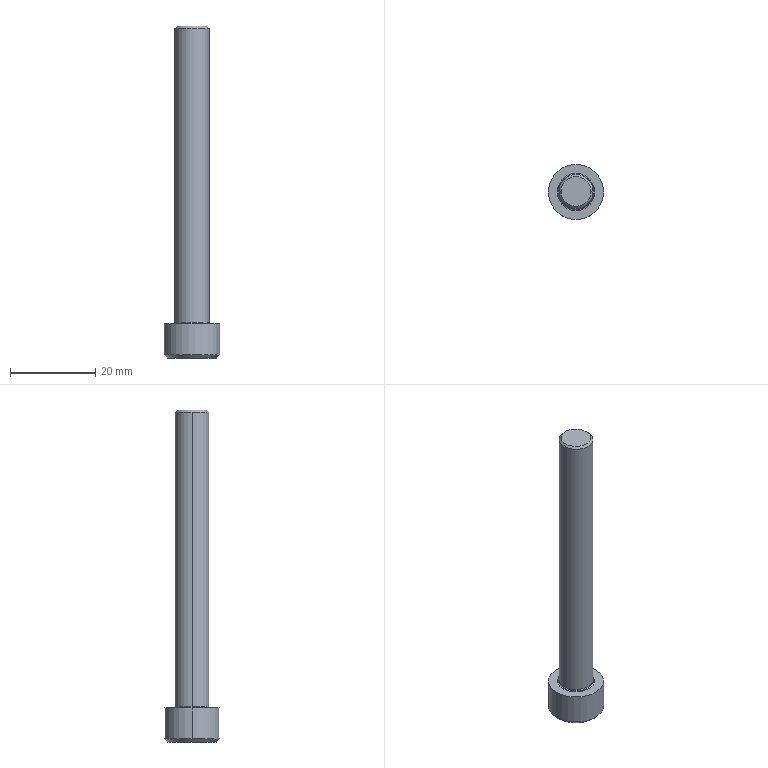Part | Creo | 1 solid | 23 faces | box 13 x 13 x 78 mm | volume 4417 mm3 | plane 9 | cone 6 | cylinder 4 | torus 4 | commonest cylinder face diameters 8 x2 13 x2
STEP:
#1=CARTESIAN_POINT('',(0.,0.,0.));
#2=DIRECTION('',(0.,0.,1.));
#3=DIRECTION('',(1.,0.,0.));
#4=AXIS2_PLACEMENT_3D('',#1,#2,#3);
#5=CARTESIAN_POINT('',(-18.464,-45.,-115.5));
#6=VERTEX_POINT('',#5);
#7=CARTESIAN_POINT('',(-16.732,-42.,-115.5));
#8=VERTEX_POINT('',#7);
#9=CARTESIAN_POINT('',(-18.464,-45.,-115.5));
#10=CARTESIAN_POINT('',(-18.409,-44.904,-115.468));
#11=CARTESIAN_POINT('',(-18.3,-44.716,-115.41));
#12=CARTESIAN_POINT('',(-18.143,-44.444,-115.34));
#13=CARTESIAN_POINT('',(-17.988,-44.176,-115.287));
#14=CARTESIAN_POINT('',(-17.834,-43.908,-115.25));
#15=CARTESIAN_POINT('',(-17.677,-43.636,-115.231));
#16=CARTESIAN_POINT('',(-17.519,-43.364,-115.231));
#17=CARTESIAN_POINT('',(-17.362,-43.092,-115.25));
#18=CARTESIAN_POINT('',(-17.208,-42.824,-115.287));
#19=CARTESIAN_POINT('',(-17.053,-42.556,-115.34));
#20=CARTESIAN_POINT('',(-16.896,-42.284,-115.41));
#21=CARTESIAN_POINT('',(-16.787,-42.096,-115.468));
#22=CARTESIAN_POINT('',(-16.732,-42.,-115.5));
#23=B_SPLINE_CURVE_WITH_KNOTS('',3,(#9,#10,#11,#12,#13,#14,#15,#16,#17,#18,#19,#20,#21,#22),.UNSPECIFIED.,.F.,.F.,(4,1,1,1,1,1,1,1,1,1,1,4),(0.,0.09091,0.1818,0.2727,0.3636,0.4545,0.5455,0.6364,0.7273,0.8182,0.9091,1.),.UNSPECIFIED.);
#24=EDGE_CURVE('',#6,#8,#23,.T.);
#25=ORIENTED_EDGE('',*,*,#24,.F.);
#26=CARTESIAN_POINT('',(-15.,-45.,-113.5));
#27=VERTEX_POINT('',#26);
#28=CARTESIAN_POINT('',(-15.,-45.,-113.5));
#29=DIRECTION('',(-0.866,0.,-0.5));
#30=VECTOR('',#29,4.);
#31=LINE('',#28,#30);
#32=EDGE_CURVE('',#27,#6,#31,.T.);
#33=ORIENTED_EDGE('',*,*,#32,.F.);
#34=CARTESIAN_POINT('',(-11.536,-45.,-115.5));
#35=VERTEX_POINT('',#34);
#36=CARTESIAN_POINT('',(-15.,-45.,-113.5));
#37=DIRECTION('',(0.866,0.,-0.5));
#38=VECTOR('',#37,4.);
#39=LINE('',#36,#38);
#40=EDGE_CURVE('',#27,#35,#39,.T.);
#41=ORIENTED_EDGE('',*,*,#40,.T.);
#42=CARTESIAN_POINT('',(-13.268,-42.,-115.5));
#43=VERTEX_POINT('',#42);
#44=CARTESIAN_POINT('',(-13.268,-42.,-115.5));
#45=CARTESIAN_POINT('',(-13.213,-42.096,-115.468));
#46=CARTESIAN_POINT('',(-13.104,-42.284,-115.41));
#47=CARTESIAN_POINT('',(-12.947,-42.556,-115.34));
#48=CARTESIAN_POINT('',(-12.792,-42.824,-115.287));
#49=CARTESIAN_POINT('',(-12.638,-43.092,-115.25));
#50=CARTESIAN_POINT('',(-12.481,-43.364,-115.231));
#51=CARTESIAN_POINT('',(-12.323,-43.636,-115.231));
#52=CARTESIAN_POINT('',(-12.166,-43.908,-115.25));
#53=CARTESIAN_POINT('',(-12.012,-44.176,-115.287));
#54=CARTESIAN_POINT('',(-11.857,-44.444,-115.34));
#55=CARTESIAN_POINT('',(-11.7,-44.716,-115.41));
#56=CARTESIAN_POINT('',(-11.591,-44.904,-115.468));
#57=CARTESIAN_POINT('',(-11.536,-45.,-115.5));
#58=B_SPLINE_CURVE_WITH_KNOTS('',3,(#44,#45,#46,#47,#48,#49,#50,#51,#52,#53,#54,#55,#56,#57),.UNSPECIFIED.,.F.,.F.,(4,1,1,1,1,1,1,1,1,1,1,4),(0.,0.09091,0.1818,0.2727,0.3636,0.4545,0.5455,0.6364,0.7273,0.8182,0.9091,1.),.UNSPECIFIED.);
#59=EDGE_CURVE('',#43,#35,#58,.T.);
#60=ORIENTED_EDGE('',*,*,#59,.F.);
#61=CARTESIAN_POINT('',(-16.732,-42.,-115.5));
#62=CARTESIAN_POINT('',(-16.622,-42.,-115.468));
#63=CARTESIAN_POINT('',(-16.404,-42.,-115.41));
#64=CARTESIAN_POINT('',(-16.091,-42.,-115.34));
#65=CARTESIAN_POINT('',(-15.782,-42.,-115.287));
#66=CARTESIAN_POINT('',(-15.472,-42.,-115.25));
#67=CARTESIAN_POINT('',(-15.158,-42.,-115.231));
#68=CARTESIAN_POINT('',(-14.842,-42.,-115.231));
#69=CARTESIAN_POINT('',(-14.528,-42.,-115.25));
#70=CARTESIAN_POINT('',(-14.218,-42.,-115.287));
#71=CARTESIAN_POINT('',(-13.909,-42.,-115.34));
#72=CARTESIAN_POINT('',(-13.596,-42.,-115.41));
#73=CARTESIAN_POINT('',(-13.378,-42.,-115.468));
#74=CARTESIAN_POINT('',(-13.268,-42.,-115.5));
#75=B_SPLINE_CURVE_WITH_KNOTS('',3,(#61,#62,#63,#64,#65,#66,#67,#68,#69,#70,#71,#72,#73,#74),.UNSPECIFIED.,.F.,.F.,(4,1,1,1,1,1,1,1,1,1,1,4),(0.,0.09091,0.1818,0.2727,0.3636,0.4545,0.5455,0.6364,0.7273,0.8182,0.9091,1.),.UNSPECIFIED.);
#76=EDGE_CURVE('',#8,#43,#75,.T.);
#77=ORIENTED_EDGE('',*,*,#76,.F.);
#78=EDGE_LOOP('',(#25,#33,#41,#60,#77));
#79=FACE_OUTER_BOUND('',#78,.F.);
#80=CARTESIAN_POINT('',(-15.,-45.,-114.524));
#81=DIRECTION('',(0.,0.,-1.));
#82=DIRECTION('',(-1.,0.,0.));
#83=AXIS2_PLACEMENT_3D('',#80,#81,#82);
#84=CONICAL_SURFACE('',#83,1.774,60.);
#85=ADVANCED_FACE('',(#79),#84,.F.);
#86=CARTESIAN_POINT('',(-16.732,-42.,-119.5));
#87=VERTEX_POINT('',#86);
#88=CARTESIAN_POINT('',(-18.464,-45.,-119.5));
#89=VERTEX_POINT('',#88);
#90=CARTESIAN_POINT('',(-16.732,-42.,-119.5));
#91=DIRECTION('',(-0.5,-0.866,0.));
#92=VECTOR('',#91,3.464);
#93=LINE('',#90,#92);
#94=EDGE_CURVE('',#87,#89,#93,.T.);
#95=ORIENTED_EDGE('',*,*,#94,.T.);
#96=CARTESIAN_POINT('',(-18.464,-45.,-119.5));
#97=DIRECTION('',(0.,0.,1.));
#98=VECTOR('',#97,4.);
#99=LINE('',#96,#98);
#100=EDGE_CURVE('',#89,#6,#99,.T.);
#101=ORIENTED_EDGE('',*,*,#100,.T.);
#102=ORIENTED_EDGE('',*,*,#24,.T.);
#103=CARTESIAN_POINT('',(-16.732,-42.,-119.5));
#104=DIRECTION('',(0.,0.,1.));
#105=VECTOR('',#104,4.);
#106=LINE('',#103,#105);
#107=EDGE_CURVE('',#87,#8,#106,.T.);
#108=ORIENTED_EDGE('',*,*,#107,.F.);
#109=EDGE_LOOP('',(#95,#101,#102,#108));
#110=FACE_OUTER_BOUND('',#109,.F.);
#111=CARTESIAN_POINT('',(-16.732,-42.,-115.5));
#112=DIRECTION('',(0.866,-0.5,0.));
#113=DIRECTION('',(-0.5,-0.866,0.));
#114=AXIS2_PLACEMENT_3D('',#111,#112,#113);
#115=PLANE('',#114);
#116=ADVANCED_FACE('',(#110),#115,.T.);
#117=CARTESIAN_POINT('',(-20.7,-45.,-119.5));
#118=VERTEX_POINT('',#117);
#119=CARTESIAN_POINT('',(-9.3,-45.,-119.5));
#120=VERTEX_POINT('',#119);
#121=CARTESIAN_POINT('',(-15.,-45.,-119.5));
#122=DIRECTION('',(0.,0.,-1.));
#123=DIRECTION('',(-1.,0.,0.));
#124=AXIS2_PLACEMENT_3D('',#121,#122,#123);
#125=CIRCLE('',#124,5.7);
#126=EDGE_CURVE('',#118,#120,#125,.T.);
#127=ORIENTED_EDGE('',*,*,#126,.F.);
#128=CARTESIAN_POINT('',(-15.,-45.,-119.5));
#129=DIRECTION('',(0.,0.,-1.));
#130=DIRECTION('',(1.,0.,0.));
#131=AXIS2_PLACEMENT_3D('',#128,#129,#130);
#132=CIRCLE('',#131,5.7);
#133=EDGE_CURVE('',#120,#118,#132,.T.);
#134=ORIENTED_EDGE('',*,*,#133,.F.);
#135=EDGE_LOOP('',(#127,#134));
#136=FACE_OUTER_BOUND('',#135,.F.);
#137=CARTESIAN_POINT('',(-16.732,-48.,-119.5));
#138=VERTEX_POINT('',#137);
#139=CARTESIAN_POINT('',(-18.464,-45.,-119.5));
#140=DIRECTION('',(0.5,-0.866,0.));
#141=VECTOR('',#140,3.464);
#142=LINE('',#139,#141);
#143=EDGE_CURVE('',#89,#138,#142,.T.);
#144=ORIENTED_EDGE('',*,*,#143,.F.);
#145=ORIENTED_EDGE('',*,*,#94,.F.);
#146=CARTESIAN_POINT('',(-13.268,-42.,-119.5));
#147=VERTEX_POINT('',#146);
#148=CARTESIAN_POINT('',(-16.732,-42.,-119.5));
#149=DIRECTION('',(1.,0.,0.));
#150=VECTOR('',#149,3.464);
#151=LINE('',#148,#150);
#152=EDGE_CURVE('',#87,#147,#151,.T.);
#153=ORIENTED_EDGE('',*,*,#152,.T.);
#154=CARTESIAN_POINT('',(-11.536,-45.,-119.5));
#155=VERTEX_POINT('',#154);
#156=CARTESIAN_POINT('',(-11.536,-45.,-119.5));
#157=DIRECTION('',(-0.5,0.866,0.));
#158=VECTOR('',#157,3.464);
#159=LINE('',#156,#158);
#160=EDGE_CURVE('',#155,#147,#159,.T.);
#161=ORIENTED_EDGE('',*,*,#160,.F.);
#162=CARTESIAN_POINT('',(-13.268,-48.,-119.5));
#163=VERTEX_POINT('',#162);
#164=CARTESIAN_POINT('',(-13.268,-48.,-119.5));
#165=DIRECTION('',(0.5,0.866,0.));
#166=VECTOR('',#165,3.464);
#167=LINE('',#164,#166);
#168=EDGE_CURVE('',#163,#155,#167,.T.);
#169=ORIENTED_EDGE('',*,*,#168,.F.);
#170=CARTESIAN_POINT('',(-13.268,-48.,-119.5));
#171=DIRECTION('',(-1.,0.,0.));
#172=VECTOR('',#171,3.464);
#173=LINE('',#170,#172);
#174=EDGE_CURVE('',#163,#138,#173,.T.);
#175=ORIENTED_EDGE('',*,*,#174,.T.);
#176=EDGE_LOOP('',(#144,#145,#153,#161,#169,#175));
#177=FACE_BOUND('',#176,.F.);
#178=CARTESIAN_POINT('',(-15.,-45.,-119.5));
#179=DIRECTION('',(0.,0.,-1.));
#180=DIRECTION('',(-1.,0.,0.));
#181=AXIS2_PLACEMENT_3D('',#178,#179,#180);
#182=PLANE('',#181);
#183=ADVANCED_FACE('',(#136,#177),#182,.T.);
#184=CARTESIAN_POINT('',(-21.5,-45.,-118.7));
#185=VERTEX_POINT('',#184);
#186=CARTESIAN_POINT('',(-8.5,-45.,-118.7));
#187=VERTEX_POINT('',#186);
#188=CARTESIAN_POINT('',(-15.,-45.,-118.7));
#189=DIRECTION('',(0.,0.,-1.));
#190=DIRECTION('',(-1.,0.,0.));
#191=AXIS2_PLACEMENT_3D('',#188,#189,#190);
#192=CIRCLE('',#191,6.5);
#193=EDGE_CURVE('',#185,#187,#192,.T.);
#194=ORIENTED_EDGE('',*,*,#193,.F.);
#195=CARTESIAN_POINT('',(-20.7,-45.,-119.5));
#196=DIRECTION('',(-0.7071,0.,0.7071));
#197=VECTOR('',#196,1.131);
#198=LINE('',#195,#197);
#199=EDGE_CURVE('',#118,#185,#198,.T.);
#200=ORIENTED_EDGE('',*,*,#199,.F.);
#201=ORIENTED_EDGE('',*,*,#126,.T.);
#202=CARTESIAN_POINT('',(-9.3,-45.,-119.5));
#203=DIRECTION('',(0.7071,0.,0.7071));
#204=VECTOR('',#203,1.131);
#205=LINE('',#202,#204);
#206=EDGE_CURVE('',#120,#187,#205,.T.);
#207=ORIENTED_EDGE('',*,*,#206,.T.);
#208=EDGE_LOOP('',(#194,#200,#201,#207));
#209=FACE_OUTER_BOUND('',#208,.F.);
#210=CARTESIAN_POINT('',(-15.,-45.,-119.1));
#211=DIRECTION('',(0.,0.,1.));
#212=DIRECTION('',(1.,0.,0.));
#213=AXIS2_PLACEMENT_3D('',#210,#211,#212);
#214=CONICAL_SURFACE('',#213,6.1,45.);
#215=ADVANCED_FACE('',(#209),#214,.T.);
#216=ORIENTED_EDGE('',*,*,#193,.T.);
#217=CARTESIAN_POINT('',(-8.5,-45.,-111.5));
#218=VERTEX_POINT('',#217);
#219=CARTESIAN_POINT('',(-8.5,-45.,-111.5));
#220=DIRECTION('',(0.,0.,-1.));
#221=VECTOR('',#220,7.2);
#222=LINE('',#219,#221);
#223=EDGE_CURVE('',#218,#187,#222,.T.);
#224=ORIENTED_EDGE('',*,*,#223,.F.);
#225=CARTESIAN_POINT('',(-21.5,-45.,-111.5));
#226=VERTEX_POINT('',#225);
#227=CARTESIAN_POINT('',(-15.,-45.,-111.5));
#228=DIRECTION('',(0.,0.,1.));
#229=DIRECTION('',(1.,0.,0.));
#230=AXIS2_PLACEMENT_3D('',#227,#228,#229);
#231=CIRCLE('',#230,6.5);
#232=EDGE_CURVE('',#218,#226,#231,.T.);
#233=ORIENTED_EDGE('',*,*,#232,.T.);
#234=CARTESIAN_POINT('',(-21.5,-45.,-111.5));
#235=DIRECTION('',(0.,0.,-1.));
#236=VECTOR('',#235,7.2);
#237=LINE('',#234,#236);
#238=EDGE_CURVE('',#226,#185,#237,.T.);
#239=ORIENTED_EDGE('',*,*,#238,.T.);
#240=EDGE_LOOP('',(#216,#224,#233,#239));
#241=FACE_OUTER_BOUND('',#240,.F.);
#242=CARTESIAN_POINT('',(-15.,-45.,-111.5));
#243=DIRECTION('',(0.,0.,-1.));
#244=DIRECTION('',(-1.,0.,0.));
#245=AXIS2_PLACEMENT_3D('',#242,#243,#244);
#246=CYLINDRICAL_SURFACE('',#245,6.5);
#247=ADVANCED_FACE('',(#241),#246,.T.);
#248=CARTESIAN_POINT('',(-15.,-45.,-118.7));
#249=DIRECTION('',(0.,0.,-1.));
#250=DIRECTION('',(1.,0.,0.));
#251=AXIS2_PLACEMENT_3D('',#248,#249,#250);
#252=CIRCLE('',#251,6.5);
#253=EDGE_CURVE('',#187,#185,#252,.T.);
#254=ORIENTED_EDGE('',*,*,#253,.T.);
#255=ORIENTED_EDGE('',*,*,#238,.F.);
#256=CARTESIAN_POINT('',(-15.,-45.,-111.5));
#257=DIRECTION('',(0.,0.,1.));
#258=DIRECTION('',(-1.,0.,0.));
#259=AXIS2_PLACEMENT_3D('',#256,#257,#258);
#260=CIRCLE('',#259,6.5);
#261=EDGE_CURVE('',#226,#218,#260,.T.);
#262=ORIENTED_EDGE('',*,*,#261,.T.);
#263=ORIENTED_EDGE('',*,*,#223,.T.);
#264=EDGE_LOOP('',(#254,#255,#262,#263));
#265=FACE_OUTER_BOUND('',#264,.F.);
#266=CARTESIAN_POINT('',(-15.,-45.,-111.5));
#267=DIRECTION('',(0.,0.,-1.));
#268=DIRECTION('',(-1.,0.,0.));
#269=AXIS2_PLACEMENT_3D('',#266,#267,#268);
#270=CYLINDRICAL_SURFACE('',#269,6.5);
#271=ADVANCED_FACE('',(#265),#270,.T.);
#272=ORIENTED_EDGE('',*,*,#253,.F.);
#273=ORIENTED_EDGE('',*,*,#206,.F.);
#274=ORIENTED_EDGE('',*,*,#133,.T.);
#275=ORIENTED_EDGE('',*,*,#199,.T.);
#276=EDGE_LOOP('',(#272,#273,#274,#275));
#277=FACE_OUTER_BOUND('',#276,.F.);
#278=CARTESIAN_POINT('',(-15.,-45.,-119.1));
#279=DIRECTION('',(0.,0.,1.));
#280=DIRECTION('',(1.,0.,0.));
#281=AXIS2_PLACEMENT_3D('',#278,#279,#280);
#282=CONICAL_SURFACE('',#281,6.1,45.);
#283=ADVANCED_FACE('',(#277),#282,.T.);
#284=ORIENTED_EDGE('',*,*,#261,.F.);
#285=ORIENTED_EDGE('',*,*,#232,.F.);
#286=EDGE_LOOP('',(#284,#285));
#287=FACE_OUTER_BOUND('',#286,.F.);
#288=CARTESIAN_POINT('',(-19.4,-45.,-111.5));
#289=VERTEX_POINT('',#288);
#290=CARTESIAN_POINT('',(-10.6,-45.,-111.5));
#291=VERTEX_POINT('',#290);
#292=CARTESIAN_POINT('',(-15.,-45.,-111.5));
#293=DIRECTION('',(0.,0.,-1.));
#294=DIRECTION('',(-1.,0.,0.));
#295=AXIS2_PLACEMENT_3D('',#292,#293,#294);
#296=CIRCLE('',#295,4.4);
#297=EDGE_CURVE('',#289,#291,#296,.T.);
#298=ORIENTED_EDGE('',*,*,#297,.F.);
#299=CARTESIAN_POINT('',(-15.,-45.,-111.5));
#300=DIRECTION('',(0.,0.,-1.));
#301=DIRECTION('',(1.,0.,0.));
#302=AXIS2_PLACEMENT_3D('',#299,#300,#301);
#303=CIRCLE('',#302,4.4);
#304=EDGE_CURVE('',#291,#289,#303,.T.);
#305=ORIENTED_EDGE('',*,*,#304,.F.);
#306=EDGE_LOOP('',(#298,#305));
#307=FACE_BOUND('',#306,.F.);
#308=CARTESIAN_POINT('',(-15.,-45.,-111.5));
#309=DIRECTION('',(0.,0.,-1.));
#310=DIRECTION('',(-1.,0.,0.));
#311=AXIS2_PLACEMENT_3D('',#308,#309,#310);
#312=PLANE('',#311);
#313=ADVANCED_FACE('',(#287,#307),#312,.F.);
#314=ORIENTED_EDGE('',*,*,#297,.T.);
#315=CARTESIAN_POINT('',(-10.883,-45.,-111.383));
#316=VERTEX_POINT('',#315);
#317=CARTESIAN_POINT('',(-10.6,-45.,-111.1));
#318=DIRECTION('',(0.,1.,0.));
#319=DIRECTION('',(0.,0.,-1.));
#320=AXIS2_PLACEMENT_3D('',#317,#318,#319);
#321=CIRCLE('',#320,0.4);
#322=EDGE_CURVE('',#291,#316,#321,.T.);
#323=ORIENTED_EDGE('',*,*,#322,.T.);
#324=CARTESIAN_POINT('',(-19.117,-45.,-111.383));
#325=VERTEX_POINT('',#324);
#326=CARTESIAN_POINT('',(-15.,-45.,-111.383));
#327=DIRECTION('',(0.,0.,-1.));
#328=DIRECTION('',(-1.,0.,0.));
#329=AXIS2_PLACEMENT_3D('',#326,#327,#328);
#330=CIRCLE('',#329,4.117);
#331=EDGE_CURVE('',#325,#316,#330,.T.);
#332=ORIENTED_EDGE('',*,*,#331,.F.);
#333=CARTESIAN_POINT('',(-19.4,-45.,-111.1));
#334=DIRECTION('',(0.,-1.,0.));
#335=DIRECTION('',(0.,0.,-1.));
#336=AXIS2_PLACEMENT_3D('',#333,#334,#335);
#337=CIRCLE('',#336,0.4);
#338=EDGE_CURVE('',#289,#325,#337,.T.);
#339=ORIENTED_EDGE('',*,*,#338,.F.);
#340=EDGE_LOOP('',(#314,#323,#332,#339));
#341=FACE_OUTER_BOUND('',#340,.F.);
#342=CARTESIAN_POINT('',(-15.,-45.,-111.1));
#343=DIRECTION('',(0.,0.,-1.));
#344=DIRECTION('',(-1.,0.,0.));
#345=AXIS2_PLACEMENT_3D('',#342,#343,#344);
#346=TOROIDAL_SURFACE('',#345,4.4,0.4);
#347=ADVANCED_FACE('',(#341),#346,.F.);
#348=ORIENTED_EDGE('',*,*,#304,.T.);
#349=ORIENTED_EDGE('',*,*,#338,.T.);
#350=CARTESIAN_POINT('',(-15.,-45.,-111.383));
#351=DIRECTION('',(0.,0.,-1.));
#352=DIRECTION('',(1.,0.,0.));
#353=AXIS2_PLACEMENT_3D('',#350,#351,#352);
#354=CIRCLE('',#353,4.117);
#355=EDGE_CURVE('',#316,#325,#354,.T.);
#356=ORIENTED_EDGE('',*,*,#355,.F.);
#357=ORIENTED_EDGE('',*,*,#322,.F.);
#358=EDGE_LOOP('',(#348,#349,#356,#357));
#359=FACE_OUTER_BOUND('',#358,.F.);
#360=CARTESIAN_POINT('',(-15.,-45.,-111.1));
#361=DIRECTION('',(0.,0.,-1.));
#362=DIRECTION('',(-1.,0.,0.));
#363=AXIS2_PLACEMENT_3D('',#360,#361,#362);
#364=TOROIDAL_SURFACE('',#363,4.4,0.4);
#365=ADVANCED_FACE('',(#359),#364,.F.);
#366=CARTESIAN_POINT('',(-11.,-45.,-111.1));
#367=VERTEX_POINT('',#366);
#368=CARTESIAN_POINT('',(-19.,-45.,-111.1));
#369=VERTEX_POINT('',#368);
#370=CARTESIAN_POINT('',(-15.,-45.,-111.1));
#371=DIRECTION('',(0.,0.,-1.));
#372=DIRECTION('',(1.,0.,0.));
#373=AXIS2_PLACEMENT_3D('',#370,#371,#372);
#374=CIRCLE('',#373,4.);
#375=EDGE_CURVE('',#367,#369,#374,.T.);
#376=ORIENTED_EDGE('',*,*,#375,.F.);
#377=CARTESIAN_POINT('',(-10.6,-45.,-111.1));
#378=DIRECTION('',(0.,1.,0.));
#379=DIRECTION('',(-0.7071,0.,-0.7071));
#380=AXIS2_PLACEMENT_3D('',#377,#378,#379);
#381=CIRCLE('',#380,0.4);
#382=EDGE_CURVE('',#316,#367,#381,.T.);
#383=ORIENTED_EDGE('',*,*,#382,.F.);
#384=ORIENTED_EDGE('',*,*,#355,.T.);
#385=CARTESIAN_POINT('',(-19.4,-45.,-111.1));
#386=DIRECTION('',(0.,-1.,0.));
#387=DIRECTION('',(0.7071,0.,-0.7071));
#388=AXIS2_PLACEMENT_3D('',#385,#386,#387);
#389=CIRCLE('',#388,0.4);
#390=EDGE_CURVE('',#325,#369,#389,.T.);
#391=ORIENTED_EDGE('',*,*,#390,.T.);
#392=EDGE_LOOP('',(#376,#383,#384,#391));
#393=FACE_OUTER_BOUND('',#392,.F.);
#394=CARTESIAN_POINT('',(-15.,-45.,-111.1));
#395=DIRECTION('',(0.,0.,-1.));
#396=DIRECTION('',(-1.,0.,0.));
#397=AXIS2_PLACEMENT_3D('',#394,#395,#396);
#398=TOROIDAL_SURFACE('',#397,4.4,0.4);
#399=ADVANCED_FACE('',(#393),#398,.F.);
#400=CARTESIAN_POINT('',(-19.,-45.,-42.));
#401=VERTEX_POINT('',#400);
#402=CARTESIAN_POINT('',(-11.,-45.,-42.));
#403=VERTEX_POINT('',#402);
#404=CARTESIAN_POINT('',(-15.,-45.,-42.));
#405=DIRECTION('',(0.,0.,1.));
#406=DIRECTION('',(-1.,0.,0.));
#407=AXIS2_PLACEMENT_3D('',#404,#405,#406);
#408=CIRCLE('',#407,4.);
#409=EDGE_CURVE('',#401,#403,#408,.T.);
#410=ORIENTED_EDGE('',*,*,#409,.T.);
#411=CARTESIAN_POINT('',(-11.,-45.,-42.));
#412=DIRECTION('',(0.,0.,-1.));
#413=VECTOR('',#412,69.1);
#414=LINE('',#411,#413);
#415=EDGE_CURVE('',#403,#367,#414,.T.);
#416=ORIENTED_EDGE('',*,*,#415,.T.);
#417=ORIENTED_EDGE('',*,*,#375,.T.);
#418=CARTESIAN_POINT('',(-19.,-45.,-42.));
#419=DIRECTION('',(0.,0.,-1.));
#420=VECTOR('',#419,69.1);
#421=LINE('',#418,#420);
#422=EDGE_CURVE('',#401,#369,#421,.T.);
#423=ORIENTED_EDGE('',*,*,#422,.F.);
#424=EDGE_LOOP('',(#410,#416,#417,#423));
#425=FACE_OUTER_BOUND('',#424,.F.);
#426=CARTESIAN_POINT('',(-15.,-45.,-41.5));
#427=DIRECTION('',(0.,0.,-1.));
#428=DIRECTION('',(-1.,0.,0.));
#429=AXIS2_PLACEMENT_3D('',#426,#427,#428);
#430=CYLINDRICAL_SURFACE('',#429,4.);
#431=ADVANCED_FACE('',(#425),#430,.T.);
#432=CARTESIAN_POINT('',(-18.5,-45.,-41.5));
#433=VERTEX_POINT('',#432);
#434=CARTESIAN_POINT('',(-11.5,-45.,-41.5));
#435=VERTEX_POINT('',#434);
#436=CARTESIAN_POINT('',(-15.,-45.,-41.5));
#437=DIRECTION('',(0.,0.,1.));
#438=DIRECTION('',(-1.,0.,0.));
#439=AXIS2_PLACEMENT_3D('',#436,#437,#438);
#440=CIRCLE('',#439,3.5);
#441=EDGE_CURVE('',#433,#435,#440,.T.);
#442=ORIENTED_EDGE('',*,*,#441,.T.);
#443=CARTESIAN_POINT('',(-11.5,-45.,-41.5));
#444=DIRECTION('',(0.7071,0.,-0.7071));
#445=VECTOR('',#444,0.7071);
#446=LINE('',#443,#445);
#447=EDGE_CURVE('',#435,#403,#446,.T.);
#448=ORIENTED_EDGE('',*,*,#447,.T.);
#449=ORIENTED_EDGE('',*,*,#409,.F.);
#450=CARTESIAN_POINT('',(-18.5,-45.,-41.5));
#451=DIRECTION('',(-0.7071,0.,-0.7071));
#452=VECTOR('',#451,0.7071);
#453=LINE('',#450,#452);
#454=EDGE_CURVE('',#433,#401,#453,.T.);
#455=ORIENTED_EDGE('',*,*,#454,.F.);
#456=EDGE_LOOP('',(#442,#448,#449,#455));
#457=FACE_OUTER_BOUND('',#456,.F.);
#458=CARTESIAN_POINT('',(-15.,-45.,-41.75));
#459=DIRECTION('',(0.,0.,-1.));
#460=DIRECTION('',(-1.,0.,0.));
#461=AXIS2_PLACEMENT_3D('',#458,#459,#460);
#462=CONICAL_SURFACE('',#461,3.75,45.);
#463=ADVANCED_FACE('',(#457),#462,.T.);
#464=ORIENTED_EDGE('',*,*,#441,.F.);
#465=CARTESIAN_POINT('',(-15.,-45.,-41.5));
#466=DIRECTION('',(0.,0.,1.));
#467=DIRECTION('',(1.,0.,0.));
#468=AXIS2_PLACEMENT_3D('',#465,#466,#467);
#469=CIRCLE('',#468,3.5);
#470=EDGE_CURVE('',#435,#433,#469,.T.);
#471=ORIENTED_EDGE('',*,*,#470,.F.);
#472=EDGE_LOOP('',(#464,#471));
#473=FACE_OUTER_BOUND('',#472,.F.);
#474=CARTESIAN_POINT('',(-15.,-45.,-41.5));
#475=DIRECTION('',(0.,0.,-1.));
#476=DIRECTION('',(-1.,0.,0.));
#477=AXIS2_PLACEMENT_3D('',#474,#475,#476);
#478=PLANE('',#477);
#479=ADVANCED_FACE('',(#473),#478,.F.);
#480=ORIENTED_EDGE('',*,*,#470,.T.);
#481=ORIENTED_EDGE('',*,*,#454,.T.);
#482=CARTESIAN_POINT('',(-15.,-45.,-42.));
#483=DIRECTION('',(0.,0.,1.));
#484=DIRECTION('',(1.,0.,0.));
#485=AXIS2_PLACEMENT_3D('',#482,#483,#484);
#486=CIRCLE('',#485,4.);
#487=EDGE_CURVE('',#403,#401,#486,.T.);
#488=ORIENTED_EDGE('',*,*,#487,.F.);
#489=ORIENTED_EDGE('',*,*,#447,.F.);
#490=EDGE_LOOP('',(#480,#481,#488,#489));
#491=FACE_OUTER_BOUND('',#490,.F.);
#492=CARTESIAN_POINT('',(-15.,-45.,-41.75));
#493=DIRECTION('',(0.,0.,-1.));
#494=DIRECTION('',(-1.,0.,0.));
#495=AXIS2_PLACEMENT_3D('',#492,#493,#494);
#496=CONICAL_SURFACE('',#495,3.75,45.);
#497=ADVANCED_FACE('',(#491),#496,.T.);
#498=ORIENTED_EDGE('',*,*,#487,.T.);
#499=ORIENTED_EDGE('',*,*,#422,.T.);
#500=CARTESIAN_POINT('',(-15.,-45.,-111.1));
#501=DIRECTION('',(0.,0.,-1.));
#502=DIRECTION('',(-1.,0.,0.));
#503=AXIS2_PLACEMENT_3D('',#500,#501,#502);
#504=CIRCLE('',#503,4.);
#505=EDGE_CURVE('',#369,#367,#504,.T.);
#506=ORIENTED_EDGE('',*,*,#505,.T.);
#507=ORIENTED_EDGE('',*,*,#415,.F.);
#508=EDGE_LOOP('',(#498,#499,#506,#507));
#509=FACE_OUTER_BOUND('',#508,.F.);
#510=CARTESIAN_POINT('',(-15.,-45.,-41.5));
#511=DIRECTION('',(0.,0.,-1.));
#512=DIRECTION('',(-1.,0.,0.));
#513=AXIS2_PLACEMENT_3D('',#510,#511,#512);
#514=CYLINDRICAL_SURFACE('',#513,4.);
#515=ADVANCED_FACE('',(#509),#514,.T.);
#516=ORIENTED_EDGE('',*,*,#505,.F.);
#517=ORIENTED_EDGE('',*,*,#390,.F.);
#518=ORIENTED_EDGE('',*,*,#331,.T.);
#519=ORIENTED_EDGE('',*,*,#382,.T.);
#520=EDGE_LOOP('',(#516,#517,#518,#519));
#521=FACE_OUTER_BOUND('',#520,.F.);
#522=CARTESIAN_POINT('',(-15.,-45.,-111.1));
#523=DIRECTION('',(0.,0.,-1.));
#524=DIRECTION('',(-1.,0.,0.));
#525=AXIS2_PLACEMENT_3D('',#522,#523,#524);
#526=TOROIDAL_SURFACE('',#525,4.4,0.4);
#527=ADVANCED_FACE('',(#521),#526,.F.);
#528=ORIENTED_EDGE('',*,*,#143,.T.);
#529=CARTESIAN_POINT('',(-16.732,-48.,-115.5));
#530=VERTEX_POINT('',#529);
#531=CARTESIAN_POINT('',(-16.732,-48.,-119.5));
#532=DIRECTION('',(0.,0.,1.));
#533=VECTOR('',#532,4.);
#534=LINE('',#531,#533);
#535=EDGE_CURVE('',#138,#530,#534,.T.);
#536=ORIENTED_EDGE('',*,*,#535,.T.);
#537=CARTESIAN_POINT('',(-16.732,-48.,-115.5));
#538=CARTESIAN_POINT('',(-16.787,-47.904,-115.468));
#539=CARTESIAN_POINT('',(-16.896,-47.716,-115.41));
#540=CARTESIAN_POINT('',(-17.053,-47.444,-115.34));
#541=CARTESIAN_POINT('',(-17.208,-47.176,-115.287));
#542=CARTESIAN_POINT('',(-17.362,-46.908,-115.25));
#543=CARTESIAN_POINT('',(-17.519,-46.636,-115.231));
#544=CARTESIAN_POINT('',(-17.677,-46.364,-115.231));
#545=CARTESIAN_POINT('',(-17.834,-46.092,-115.25));
#546=CARTESIAN_POINT('',(-17.988,-45.824,-115.287));
#547=CARTESIAN_POINT('',(-18.143,-45.556,-115.34));
#548=CARTESIAN_POINT('',(-18.3,-45.284,-115.41));
#549=CARTESIAN_POINT('',(-18.409,-45.096,-115.468));
#550=CARTESIAN_POINT('',(-18.464,-45.,-115.5));
#551=B_SPLINE_CURVE_WITH_KNOTS('',3,(#537,#538,#539,#540,#541,#542,#543,#544,#545,#546,#547,#548,#549,#550),.UNSPECIFIED.,.F.,.F.,(4,1,1,1,1,1,1,1,1,1,1,4),(0.,0.09091,0.1818,0.2727,0.3636,0.4545,0.5455,0.6364,0.7273,0.8182,0.9091,1.),.UNSPECIFIED.);
#552=EDGE_CURVE('',#530,#6,#551,.T.);
#553=ORIENTED_EDGE('',*,*,#552,.T.);
#554=ORIENTED_EDGE('',*,*,#100,.F.);
#555=EDGE_LOOP('',(#528,#536,#553,#554));
#556=FACE_OUTER_BOUND('',#555,.F.);
#557=CARTESIAN_POINT('',(-18.464,-45.,-115.5));
#558=DIRECTION('',(0.866,0.5,0.));
#559=DIRECTION('',(0.5,-0.866,0.));
#560=AXIS2_PLACEMENT_3D('',#557,#558,#559);
#561=PLANE('',#560);
#562=ADVANCED_FACE('',(#556),#561,.T.);
#563=ORIENTED_EDGE('',*,*,#174,.F.);
#564=CARTESIAN_POINT('',(-13.268,-48.,-115.5));
#565=VERTEX_POINT('',#564);
#566=CARTESIAN_POINT('',(-13.268,-48.,-119.5));
#567=DIRECTION('',(0.,0.,1.));
#568=VECTOR('',#567,4.);
#569=LINE('',#566,#568);
#570=EDGE_CURVE('',#163,#565,#569,.T.);
#571=ORIENTED_EDGE('',*,*,#570,.T.);
#572=CARTESIAN_POINT('',(-13.268,-48.,-115.5));
#573=CARTESIAN_POINT('',(-13.378,-48.,-115.468));
#574=CARTESIAN_POINT('',(-13.596,-48.,-115.41));
#575=CARTESIAN_POINT('',(-13.909,-48.,-115.34));
#576=CARTESIAN_POINT('',(-14.218,-48.,-115.287));
#577=CARTESIAN_POINT('',(-14.528,-48.,-115.25));
#578=CARTESIAN_POINT('',(-14.842,-48.,-115.231));
#579=CARTESIAN_POINT('',(-15.158,-48.,-115.231));
#580=CARTESIAN_POINT('',(-15.472,-48.,-115.25));
#581=CARTESIAN_POINT('',(-15.782,-48.,-115.287));
#582=CARTESIAN_POINT('',(-16.091,-48.,-115.34));
#583=CARTESIAN_POINT('',(-16.404,-48.,-115.41));
#584=CARTESIAN_POINT('',(-16.622,-48.,-115.468));
#585=CARTESIAN_POINT('',(-16.732,-48.,-115.5));
#586=B_SPLINE_CURVE_WITH_KNOTS('',3,(#572,#573,#574,#575,#576,#577,#578,#579,#580,#581,#582,#583,#584,#585),.UNSPECIFIED.,.F.,.F.,(4,1,1,1,1,1,1,1,1,1,1,4),(0.,0.09091,0.1818,0.2727,0.3636,0.4545,0.5455,0.6364,0.7273,0.8182,0.9091,1.),.UNSPECIFIED.);
#587=EDGE_CURVE('',#565,#530,#586,.T.);
#588=ORIENTED_EDGE('',*,*,#587,.T.);
#589=ORIENTED_EDGE('',*,*,#535,.F.);
#590=EDGE_LOOP('',(#563,#571,#588,#589));
#591=FACE_OUTER_BOUND('',#590,.F.);
#592=CARTESIAN_POINT('',(-16.732,-48.,-115.5));
#593=DIRECTION('',(0.,1.,0.));
#594=DIRECTION('',(0.,0.,-1.));
#595=AXIS2_PLACEMENT_3D('',#592,#593,#594);
#596=PLANE('',#595);
#597=ADVANCED_FACE('',(#591),#596,.T.);
#598=ORIENTED_EDGE('',*,*,#168,.T.);
#599=CARTESIAN_POINT('',(-11.536,-45.,-119.5));
#600=DIRECTION('',(0.,0.,1.));
#601=VECTOR('',#600,4.);
#602=LINE('',#599,#601);
#603=EDGE_CURVE('',#155,#35,#602,.T.);
#604=ORIENTED_EDGE('',*,*,#603,.T.);
#605=CARTESIAN_POINT('',(-11.536,-45.,-115.5));
#606=CARTESIAN_POINT('',(-11.591,-45.096,-115.468));
#607=CARTESIAN_POINT('',(-11.7,-45.284,-115.41));
#608=CARTESIAN_POINT('',(-11.857,-45.556,-115.34));
#609=CARTESIAN_POINT('',(-12.012,-45.824,-115.287));
#610=CARTESIAN_POINT('',(-12.166,-46.092,-115.25));
#611=CARTESIAN_POINT('',(-12.323,-46.364,-115.231));
#612=CARTESIAN_POINT('',(-12.481,-46.636,-115.231));
#613=CARTESIAN_POINT('',(-12.638,-46.908,-115.25));
#614=CARTESIAN_POINT('',(-12.792,-47.176,-115.287));
#615=CARTESIAN_POINT('',(-12.947,-47.444,-115.34));
#616=CARTESIAN_POINT('',(-13.104,-47.716,-115.41));
#617=CARTESIAN_POINT('',(-13.213,-47.904,-115.468));
#618=CARTESIAN_POINT('',(-13.268,-48.,-115.5));
#619=B_SPLINE_CURVE_WITH_KNOTS('',3,(#605,#606,#607,#608,#609,#610,#611,#612,#613,#614,#615,#616,#617,#618),.UNSPECIFIED.,.F.,.F.,(4,1,1,1,1,1,1,1,1,1,1,4),(0.,0.09091,0.1818,0.2727,0.3636,0.4545,0.5455,0.6364,0.7273,0.8182,0.9091,1.),.UNSPECIFIED.);
#620=EDGE_CURVE('',#35,#565,#619,.T.);
#621=ORIENTED_EDGE('',*,*,#620,.T.);
#622=ORIENTED_EDGE('',*,*,#570,.F.);
#623=EDGE_LOOP('',(#598,#604,#621,#622));
#624=FACE_OUTER_BOUND('',#623,.F.);
#625=CARTESIAN_POINT('',(-13.268,-48.,-115.5));
#626=DIRECTION('',(-0.866,0.5,0.));
#627=DIRECTION('',(0.5,0.866,0.));
#628=AXIS2_PLACEMENT_3D('',#625,#626,#627);
#629=PLANE('',#628);
#630=ADVANCED_FACE('',(#624),#629,.T.);
#631=ORIENTED_EDGE('',*,*,#160,.T.);
#632=CARTESIAN_POINT('',(-13.268,-42.,-119.5));
#633=DIRECTION('',(0.,0.,1.));
#634=VECTOR('',#633,4.);
#635=LINE('',#632,#634);
#636=EDGE_CURVE('',#147,#43,#635,.T.);
#637=ORIENTED_EDGE('',*,*,#636,.T.);
#638=ORIENTED_EDGE('',*,*,#59,.T.);
#639=ORIENTED_EDGE('',*,*,#603,.F.);
#640=EDGE_LOOP('',(#631,#637,#638,#639));
#641=FACE_OUTER_BOUND('',#640,.F.);
#642=CARTESIAN_POINT('',(-11.536,-45.,-115.5));
#643=DIRECTION('',(-0.866,-0.5,0.));
#644=DIRECTION('',(-0.5,0.866,0.));
#645=AXIS2_PLACEMENT_3D('',#642,#643,#644);
#646=PLANE('',#645);
#647=ADVANCED_FACE('',(#641),#646,.T.);
#648=ORIENTED_EDGE('',*,*,#152,.F.);
#649=ORIENTED_EDGE('',*,*,#107,.T.);
#650=ORIENTED_EDGE('',*,*,#76,.T.);
#651=ORIENTED_EDGE('',*,*,#636,.F.);
#652=EDGE_LOOP('',(#648,#649,#650,#651));
#653=FACE_OUTER_BOUND('',#652,.F.);
#654=CARTESIAN_POINT('',(-13.268,-42.,-115.5));
#655=DIRECTION('',(0.,-1.,0.));
#656=DIRECTION('',(0.,0.,1.));
#657=AXIS2_PLACEMENT_3D('',#654,#655,#656);
#658=PLANE('',#657);
#659=ADVANCED_FACE('',(#653),#658,.T.);
#660=ORIENTED_EDGE('',*,*,#620,.F.);
#661=ORIENTED_EDGE('',*,*,#40,.F.);
#662=ORIENTED_EDGE('',*,*,#32,.T.);
#663=ORIENTED_EDGE('',*,*,#552,.F.);
#664=ORIENTED_EDGE('',*,*,#587,.F.);
#665=EDGE_LOOP('',(#660,#661,#662,#663,#664));
#666=FACE_OUTER_BOUND('',#665,.F.);
#667=CARTESIAN_POINT('',(-15.,-45.,-114.524));
#668=DIRECTION('',(0.,0.,-1.));
#669=DIRECTION('',(-1.,0.,0.));
#670=AXIS2_PLACEMENT_3D('',#667,#668,#669);
#671=CONICAL_SURFACE('',#670,1.774,60.);
#672=ADVANCED_FACE('',(#666),#671,.F.);
#673=CLOSED_SHELL('',(#85,#116,#183,#215,#247,#271,#283,#313,#347,#365,#399,#431,#463,#479,#497,#515,#527,#562,#597,#630,#647,#659,#672));
#674=MANIFOLD_SOLID_BREP('',#673);
#675=(LENGTH_UNIT()NAMED_UNIT(*)SI_UNIT(.MILLI.,.METRE.));
#676=UNCERTAINTY_MEASURE_WITH_UNIT(LENGTH_MEASURE(0.008013),#675,'','');
#677=(NAMED_UNIT(*)PLANE_ANGLE_UNIT()SI_UNIT($,.RADIAN.));
#678=PLANE_ANGLE_MEASURE_WITH_UNIT(PLANE_ANGLE_MEASURE(0.01745),#677);
#679=(CONVERSION_BASED_UNIT('DEGREE',#678)NAMED_UNIT(*)PLANE_ANGLE_UNIT());
#680=(NAMED_UNIT(*)SI_UNIT($,.STERADIAN.)SOLID_ANGLE_UNIT());
#681=(GEOMETRIC_REPRESENTATION_CONTEXT(3)GLOBAL_UNCERTAINTY_ASSIGNED_CONTEXT((#676))GLOBAL_UNIT_ASSIGNED_CONTEXT((#675,#679,#680))REPRESENTATION_CONTEXT('',''));
#682=ADVANCED_BREP_SHAPE_REPRESENTATION('',(#4,#674),#681);